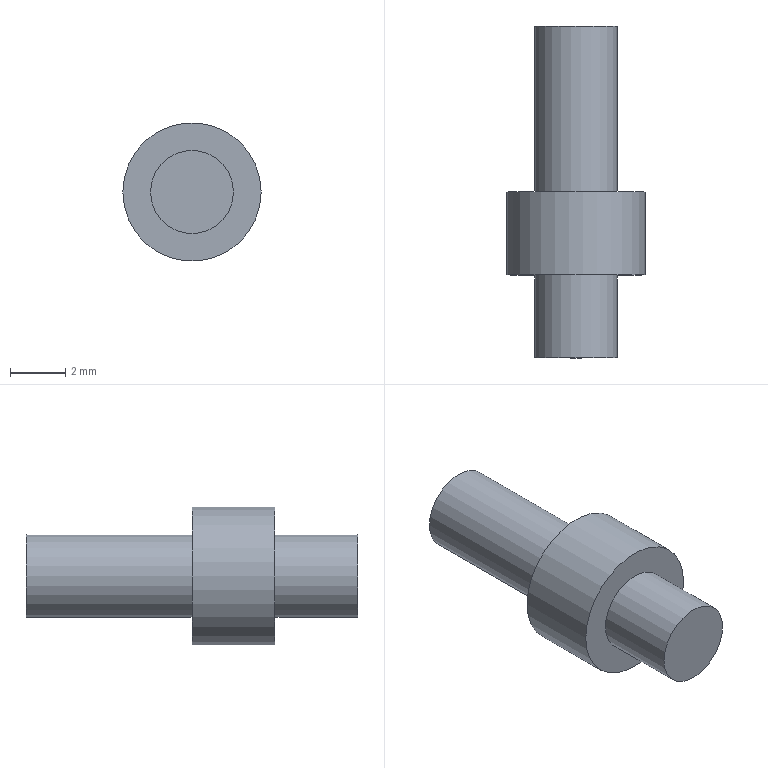Part | STEP file | 2-09.2 | 1 solid | 7 faces | box 5 x 12 x 5 mm | volume 122.522 mm3 | plane 4 | cylinder 3 | commonest cylinder face diameters 3 x2 5 x1
STEP:
#1=CARTESIAN_POINT('',(0.,0.,0.));
#2=DIRECTION('',(0.,0.,1.));
#3=DIRECTION('',(1.,0.,0.));
#4=AXIS2_PLACEMENT_3D('',#1,#2,#3);
#5=CARTESIAN_POINT('',(2.5,0.,0.));
#6=VERTEX_POINT('',#5);
#7=CARTESIAN_POINT('',(0.,0.,0.));
#8=DIRECTION('',(0.,-1.,0.));
#9=DIRECTION('',(1.,0.,0.));
#10=AXIS2_PLACEMENT_3D('',#7,#8,#9);
#11=CIRCLE('',#10,2.5);
#12=CARTESIAN_POINT('',(0.,0.,0.));
#13=DIRECTION('',(0.,-1.,0.));
#14=DIRECTION('',(1.,0.,0.));
#15=AXIS2_PLACEMENT_3D('',#12,#13,#14);
#16=CYLINDRICAL_SURFACE('',#15,2.5);
#17=CARTESIAN_POINT('',(0.,0.));
#18=DIRECTION('',(1.,0.));
#19=VECTOR('',#18,1.);
#20=LINE('',#17,#19);
#21=(GEOMETRIC_REPRESENTATION_CONTEXT(2)PARAMETRIC_REPRESENTATION_CONTEXT()REPRESENTATION_CONTEXT('',''));
#22=DEFINITIONAL_REPRESENTATION('',(#20),#21);
#23=PCURVE('',#16,#22);
#24=CARTESIAN_POINT('',(-0.6699,0.,0.));
#25=DIRECTION('',(0.,-1.,0.));
#26=DIRECTION('',(1.,0.,0.));
#27=AXIS2_PLACEMENT_3D('',#24,#25,#26);
#28=PLANE('',#27);
#29=CARTESIAN_POINT('',(0.6699,0.));
#30=DIRECTION('',(1.,0.));
#31=AXIS2_PLACEMENT_2D('',#29,#30);
#32=CIRCLE('',#31,2.5);
#33=(GEOMETRIC_REPRESENTATION_CONTEXT(2)PARAMETRIC_REPRESENTATION_CONTEXT()REPRESENTATION_CONTEXT('',''));
#34=DEFINITIONAL_REPRESENTATION('',(#32),#33);
#35=PCURVE('',#28,#34);
#36=SURFACE_CURVE('',#11,(#23,#35),.PCURVE_S1.);
#37=EDGE_CURVE('',#6,#6,#36,.T.);
#38=ORIENTED_EDGE('',*,*,#37,.T.);
#39=CARTESIAN_POINT('',(2.5,-3.,0.));
#40=VERTEX_POINT('',#39);
#41=CARTESIAN_POINT('',(2.5,0.,0.));
#42=DIRECTION('',(0.,-1.,0.));
#43=VECTOR('',#42,1.);
#44=LINE('',#41,#43);
#45=CARTESIAN_POINT('',(6.283,0.));
#46=DIRECTION('',(0.,1.));
#47=VECTOR('',#46,1.);
#48=LINE('',#45,#47);
#49=(GEOMETRIC_REPRESENTATION_CONTEXT(2)PARAMETRIC_REPRESENTATION_CONTEXT()REPRESENTATION_CONTEXT('',''));
#50=DEFINITIONAL_REPRESENTATION('',(#48),#49);
#51=PCURVE('',#16,#50);
#52=CARTESIAN_POINT('',(0.,0.));
#53=DIRECTION('',(0.,1.));
#54=VECTOR('',#53,1.);
#55=LINE('',#52,#54);
#56=(GEOMETRIC_REPRESENTATION_CONTEXT(2)PARAMETRIC_REPRESENTATION_CONTEXT()REPRESENTATION_CONTEXT('',''));
#57=DEFINITIONAL_REPRESENTATION('',(#55),#56);
#58=PCURVE('',#16,#57);
#59=SEAM_CURVE('',#44,(#51,#58),.PCURVE_S1.);
#60=EDGE_CURVE('',#6,#40,#59,.T.);
#61=ORIENTED_EDGE('',*,*,#60,.T.);
#62=CARTESIAN_POINT('',(0.,-3.,0.));
#63=DIRECTION('',(0.,-1.,0.));
#64=DIRECTION('',(1.,0.,0.));
#65=AXIS2_PLACEMENT_3D('',#62,#63,#64);
#66=CIRCLE('',#65,2.5);
#67=CARTESIAN_POINT('',(0.,3.));
#68=DIRECTION('',(1.,0.));
#69=VECTOR('',#68,1.);
#70=LINE('',#67,#69);
#71=(GEOMETRIC_REPRESENTATION_CONTEXT(2)PARAMETRIC_REPRESENTATION_CONTEXT()REPRESENTATION_CONTEXT('',''));
#72=DEFINITIONAL_REPRESENTATION('',(#70),#71);
#73=PCURVE('',#16,#72);
#74=CARTESIAN_POINT('',(-0.6699,-3.,0.));
#75=DIRECTION('',(0.,-1.,0.));
#76=DIRECTION('',(1.,0.,0.));
#77=AXIS2_PLACEMENT_3D('',#74,#75,#76);
#78=PLANE('',#77);
#79=CARTESIAN_POINT('',(0.6699,0.));
#80=DIRECTION('',(1.,0.));
#81=AXIS2_PLACEMENT_2D('',#79,#80);
#82=CIRCLE('',#81,2.5);
#83=(GEOMETRIC_REPRESENTATION_CONTEXT(2)PARAMETRIC_REPRESENTATION_CONTEXT()REPRESENTATION_CONTEXT('',''));
#84=DEFINITIONAL_REPRESENTATION('',(#82),#83);
#85=PCURVE('',#78,#84);
#86=SURFACE_CURVE('',#66,(#73,#85),.PCURVE_S1.);
#87=EDGE_CURVE('',#40,#40,#86,.T.);
#88=ORIENTED_EDGE('',*,*,#87,.F.);
#89=ORIENTED_EDGE('',*,*,#60,.F.);
#90=EDGE_LOOP('',(#38,#61,#88,#89));
#91=FACE_BOUND('',#90,.T.);
#92=ADVANCED_FACE('',(#91),#16,.T.);
#93=ORIENTED_EDGE('',*,*,#37,.T.);
#94=EDGE_LOOP('',(#93));
#95=FACE_BOUND('',#94,.F.);
#96=CARTESIAN_POINT('',(1.5,0.,0.));
#97=VERTEX_POINT('',#96);
#98=CARTESIAN_POINT('',(0.,0.,0.));
#99=DIRECTION('',(0.,-1.,0.));
#100=DIRECTION('',(1.,0.,0.));
#101=AXIS2_PLACEMENT_3D('',#98,#99,#100);
#102=CIRCLE('',#101,1.5);
#103=CARTESIAN_POINT('',(0.6699,0.));
#104=DIRECTION('',(1.,0.));
#105=AXIS2_PLACEMENT_2D('',#103,#104);
#106=CIRCLE('',#105,1.5);
#107=(GEOMETRIC_REPRESENTATION_CONTEXT(2)PARAMETRIC_REPRESENTATION_CONTEXT()REPRESENTATION_CONTEXT('',''));
#108=DEFINITIONAL_REPRESENTATION('',(#106),#107);
#109=PCURVE('',#28,#108);
#110=CARTESIAN_POINT('',(0.,0.,0.));
#111=DIRECTION('',(0.,1.,0.));
#112=DIRECTION('',(1.,0.,0.));
#113=AXIS2_PLACEMENT_3D('',#110,#111,#112);
#114=CYLINDRICAL_SURFACE('',#113,1.5);
#115=CARTESIAN_POINT('',(6.283,0.));
#116=DIRECTION('',(-1.,0.));
#117=VECTOR('',#116,1.);
#118=LINE('',#115,#117);
#119=(GEOMETRIC_REPRESENTATION_CONTEXT(2)PARAMETRIC_REPRESENTATION_CONTEXT()REPRESENTATION_CONTEXT('',''));
#120=DEFINITIONAL_REPRESENTATION('',(#118),#119);
#121=PCURVE('',#114,#120);
#122=SURFACE_CURVE('',#102,(#109,#121),.PCURVE_S1.);
#123=EDGE_CURVE('',#97,#97,#122,.T.);
#124=ORIENTED_EDGE('',*,*,#123,.F.);
#125=EDGE_LOOP('',(#124));
#126=FACE_BOUND('',#125,.F.);
#127=ADVANCED_FACE('',(#95,#126),#28,.F.);
#128=CARTESIAN_POINT('',(1.5,6.,0.));
#129=VERTEX_POINT('',#128);
#130=CARTESIAN_POINT('',(1.5,0.,0.));
#131=DIRECTION('',(0.,1.,0.));
#132=VECTOR('',#131,1.);
#133=LINE('',#130,#132);
#134=CARTESIAN_POINT('',(6.283,0.));
#135=DIRECTION('',(0.,1.));
#136=VECTOR('',#135,1.);
#137=LINE('',#134,#136);
#138=(GEOMETRIC_REPRESENTATION_CONTEXT(2)PARAMETRIC_REPRESENTATION_CONTEXT()REPRESENTATION_CONTEXT('',''));
#139=DEFINITIONAL_REPRESENTATION('',(#137),#138);
#140=PCURVE('',#114,#139);
#141=CARTESIAN_POINT('',(0.,0.));
#142=DIRECTION('',(0.,1.));
#143=VECTOR('',#142,1.);
#144=LINE('',#141,#143);
#145=(GEOMETRIC_REPRESENTATION_CONTEXT(2)PARAMETRIC_REPRESENTATION_CONTEXT()REPRESENTATION_CONTEXT('',''));
#146=DEFINITIONAL_REPRESENTATION('',(#144),#145);
#147=PCURVE('',#114,#146);
#148=SEAM_CURVE('',#133,(#140,#147),.PCURVE_S1.);
#149=EDGE_CURVE('',#97,#129,#148,.T.);
#150=ORIENTED_EDGE('',*,*,#149,.T.);
#151=CARTESIAN_POINT('',(0.,6.,0.));
#152=DIRECTION('',(0.,-1.,0.));
#153=DIRECTION('',(1.,0.,0.));
#154=AXIS2_PLACEMENT_3D('',#151,#152,#153);
#155=CIRCLE('',#154,1.5);
#156=CARTESIAN_POINT('',(6.283,6.));
#157=DIRECTION('',(-1.,0.));
#158=VECTOR('',#157,1.);
#159=LINE('',#156,#158);
#160=(GEOMETRIC_REPRESENTATION_CONTEXT(2)PARAMETRIC_REPRESENTATION_CONTEXT()REPRESENTATION_CONTEXT('',''));
#161=DEFINITIONAL_REPRESENTATION('',(#159),#160);
#162=PCURVE('',#114,#161);
#163=CARTESIAN_POINT('',(-0.4019,6.,0.));
#164=DIRECTION('',(0.,-1.,0.));
#165=DIRECTION('',(1.,0.,0.));
#166=AXIS2_PLACEMENT_3D('',#163,#164,#165);
#167=PLANE('',#166);
#168=CARTESIAN_POINT('',(0.4019,0.));
#169=DIRECTION('',(1.,0.));
#170=AXIS2_PLACEMENT_2D('',#168,#169);
#171=CIRCLE('',#170,1.5);
#172=(GEOMETRIC_REPRESENTATION_CONTEXT(2)PARAMETRIC_REPRESENTATION_CONTEXT()REPRESENTATION_CONTEXT('',''));
#173=DEFINITIONAL_REPRESENTATION('',(#171),#172);
#174=PCURVE('',#167,#173);
#175=SURFACE_CURVE('',#155,(#162,#174),.PCURVE_S1.);
#176=EDGE_CURVE('',#129,#129,#175,.T.);
#177=ORIENTED_EDGE('',*,*,#176,.T.);
#178=ORIENTED_EDGE('',*,*,#149,.F.);
#179=ORIENTED_EDGE('',*,*,#123,.F.);
#180=EDGE_LOOP('',(#150,#177,#178,#179));
#181=FACE_BOUND('',#180,.T.);
#182=ADVANCED_FACE('',(#181),#114,.T.);
#183=ORIENTED_EDGE('',*,*,#176,.T.);
#184=EDGE_LOOP('',(#183));
#185=FACE_BOUND('',#184,.F.);
#186=ADVANCED_FACE('',(#185),#167,.F.);
#187=ORIENTED_EDGE('',*,*,#87,.T.);
#188=EDGE_LOOP('',(#187));
#189=FACE_BOUND('',#188,.T.);
#190=CARTESIAN_POINT('',(1.5,-3.,0.));
#191=VERTEX_POINT('',#190);
#192=CARTESIAN_POINT('',(0.,-3.,0.));
#193=DIRECTION('',(0.,-1.,0.));
#194=DIRECTION('',(1.,0.,0.));
#195=AXIS2_PLACEMENT_3D('',#192,#193,#194);
#196=CIRCLE('',#195,1.5);
#197=CARTESIAN_POINT('',(0.6699,0.));
#198=DIRECTION('',(1.,0.));
#199=AXIS2_PLACEMENT_2D('',#197,#198);
#200=CIRCLE('',#199,1.5);
#201=(GEOMETRIC_REPRESENTATION_CONTEXT(2)PARAMETRIC_REPRESENTATION_CONTEXT()REPRESENTATION_CONTEXT('',''));
#202=DEFINITIONAL_REPRESENTATION('',(#200),#201);
#203=PCURVE('',#78,#202);
#204=CARTESIAN_POINT('',(0.,-3.,0.));
#205=DIRECTION('',(0.,-1.,0.));
#206=DIRECTION('',(1.,0.,0.));
#207=AXIS2_PLACEMENT_3D('',#204,#205,#206);
#208=CYLINDRICAL_SURFACE('',#207,1.5);
#209=CARTESIAN_POINT('',(0.,0.));
#210=DIRECTION('',(1.,0.));
#211=VECTOR('',#210,1.);
#212=LINE('',#209,#211);
#213=(GEOMETRIC_REPRESENTATION_CONTEXT(2)PARAMETRIC_REPRESENTATION_CONTEXT()REPRESENTATION_CONTEXT('',''));
#214=DEFINITIONAL_REPRESENTATION('',(#212),#213);
#215=PCURVE('',#208,#214);
#216=SURFACE_CURVE('',#196,(#203,#215),.PCURVE_S1.);
#217=EDGE_CURVE('',#191,#191,#216,.T.);
#218=ORIENTED_EDGE('',*,*,#217,.F.);
#219=EDGE_LOOP('',(#218));
#220=FACE_BOUND('',#219,.T.);
#221=ADVANCED_FACE('',(#189,#220),#78,.T.);
#222=ORIENTED_EDGE('',*,*,#217,.T.);
#223=CARTESIAN_POINT('',(1.5,-6.,0.));
#224=VERTEX_POINT('',#223);
#225=CARTESIAN_POINT('',(1.5,-3.,0.));
#226=DIRECTION('',(0.,-1.,0.));
#227=VECTOR('',#226,1.);
#228=LINE('',#225,#227);
#229=CARTESIAN_POINT('',(6.283,0.));
#230=DIRECTION('',(0.,1.));
#231=VECTOR('',#230,1.);
#232=LINE('',#229,#231);
#233=(GEOMETRIC_REPRESENTATION_CONTEXT(2)PARAMETRIC_REPRESENTATION_CONTEXT()REPRESENTATION_CONTEXT('',''));
#234=DEFINITIONAL_REPRESENTATION('',(#232),#233);
#235=PCURVE('',#208,#234);
#236=CARTESIAN_POINT('',(0.,0.));
#237=DIRECTION('',(0.,1.));
#238=VECTOR('',#237,1.);
#239=LINE('',#236,#238);
#240=(GEOMETRIC_REPRESENTATION_CONTEXT(2)PARAMETRIC_REPRESENTATION_CONTEXT()REPRESENTATION_CONTEXT('',''));
#241=DEFINITIONAL_REPRESENTATION('',(#239),#240);
#242=PCURVE('',#208,#241);
#243=SEAM_CURVE('',#228,(#235,#242),.PCURVE_S1.);
#244=EDGE_CURVE('',#191,#224,#243,.T.);
#245=ORIENTED_EDGE('',*,*,#244,.T.);
#246=CARTESIAN_POINT('',(0.,-6.,0.));
#247=DIRECTION('',(0.,-1.,0.));
#248=DIRECTION('',(1.,0.,0.));
#249=AXIS2_PLACEMENT_3D('',#246,#247,#248);
#250=CIRCLE('',#249,1.5);
#251=CARTESIAN_POINT('',(0.,3.));
#252=DIRECTION('',(1.,0.));
#253=VECTOR('',#252,1.);
#254=LINE('',#251,#253);
#255=(GEOMETRIC_REPRESENTATION_CONTEXT(2)PARAMETRIC_REPRESENTATION_CONTEXT()REPRESENTATION_CONTEXT('',''));
#256=DEFINITIONAL_REPRESENTATION('',(#254),#255);
#257=PCURVE('',#208,#256);
#258=CARTESIAN_POINT('',(-0.4019,-6.,0.));
#259=DIRECTION('',(0.,-1.,0.));
#260=DIRECTION('',(1.,0.,0.));
#261=AXIS2_PLACEMENT_3D('',#258,#259,#260);
#262=PLANE('',#261);
#263=CARTESIAN_POINT('',(0.4019,0.));
#264=DIRECTION('',(1.,0.));
#265=AXIS2_PLACEMENT_2D('',#263,#264);
#266=CIRCLE('',#265,1.5);
#267=(GEOMETRIC_REPRESENTATION_CONTEXT(2)PARAMETRIC_REPRESENTATION_CONTEXT()REPRESENTATION_CONTEXT('',''));
#268=DEFINITIONAL_REPRESENTATION('',(#266),#267);
#269=PCURVE('',#262,#268);
#270=SURFACE_CURVE('',#250,(#257,#269),.PCURVE_S1.);
#271=EDGE_CURVE('',#224,#224,#270,.T.);
#272=ORIENTED_EDGE('',*,*,#271,.F.);
#273=ORIENTED_EDGE('',*,*,#244,.F.);
#274=EDGE_LOOP('',(#222,#245,#272,#273));
#275=FACE_BOUND('',#274,.T.);
#276=ADVANCED_FACE('',(#275),#208,.T.);
#277=ORIENTED_EDGE('',*,*,#271,.T.);
#278=EDGE_LOOP('',(#277));
#279=FACE_BOUND('',#278,.T.);
#280=ADVANCED_FACE('',(#279),#262,.T.);
#281=CLOSED_SHELL('',(#92,#127,#182,#186,#221,#276,#280));
#282=MANIFOLD_SOLID_BREP('',#281);
#283=(LENGTH_UNIT()NAMED_UNIT(*)SI_UNIT(.MILLI.,.METRE.));
#284=UNCERTAINTY_MEASURE_WITH_UNIT(LENGTH_MEASURE(0.0000001),#283,'','');
#285=(NAMED_UNIT(*)PLANE_ANGLE_UNIT()SI_UNIT($,.RADIAN.));
#286=(NAMED_UNIT(*)SI_UNIT($,.STERADIAN.)SOLID_ANGLE_UNIT());
#287=(GEOMETRIC_REPRESENTATION_CONTEXT(3)GLOBAL_UNCERTAINTY_ASSIGNED_CONTEXT((#284))GLOBAL_UNIT_ASSIGNED_CONTEXT((#283,#285,#286))REPRESENTATION_CONTEXT('',''));
#288=ADVANCED_BREP_SHAPE_REPRESENTATION('',(#4,#282),#287);